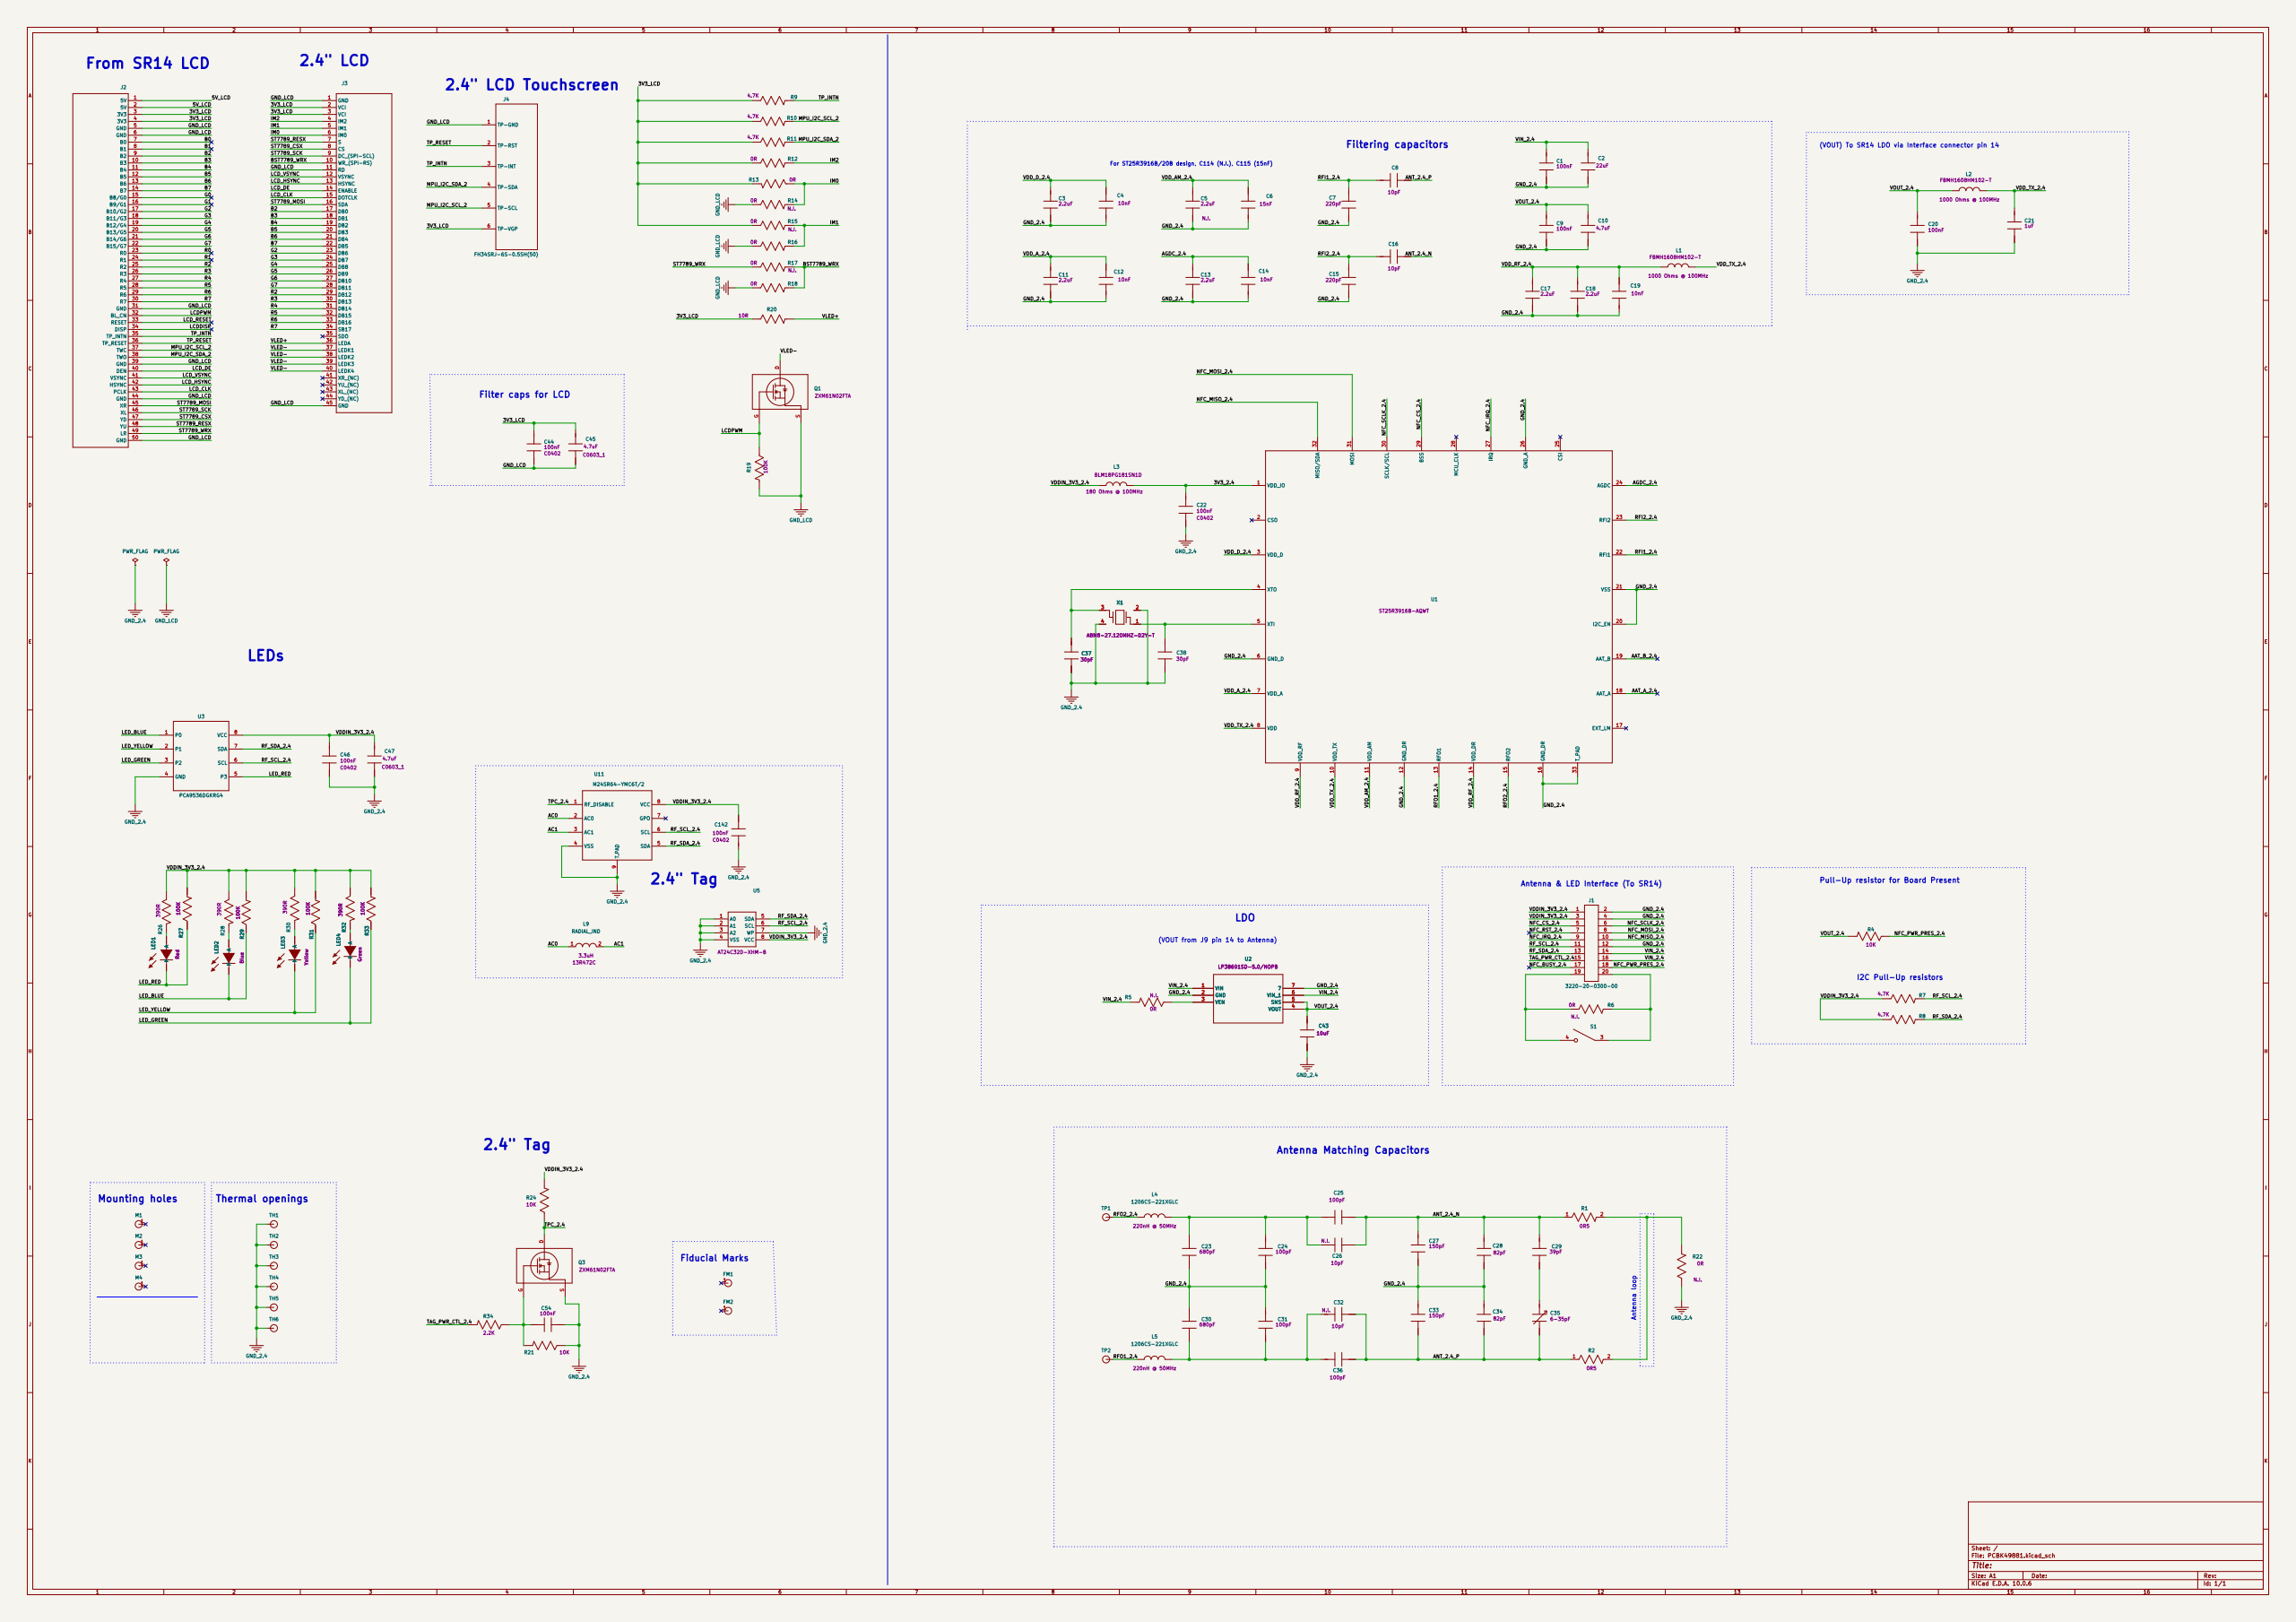Circuit board | KiCad | 113 parts | 116 nets
Bill of materials:
"Refs","Value","Footprint","Qty","DNP"
"C1,C4,C6,C7,C9,C12,C14,C15,C19-C34,C36-C38,C44,C46,C54,C142","CAP-SM","Capacitor_SMD:C_0402_1005Metric","31",""
"C2,C3,C5,C10,C11,C13,C17,C18,C43,C45,C47","CAP-SM","Capacitor_SMD:C_0603_1608Metric","11",""
"C8,C16","CAP","Capacitor_SMD:C_0402_1005Metric","2",""
"C35","TRIM_CAP","Library:TSC3S","1",""
"FM1,FM2","FM-40/80","Library:FM-40$2F$80","2",""
"J1","3220-20-0300-00","Library:3220-20-0300-00","1",""
"J2","LCM-50PIN-ANT","Library:LCD-50P-ANT","1",""
"J3","62684-452100ALF","Library:LCD-45P-0.5MM","1",""
"J4","FH34SRJ-6S-0.5SH(50)","Library:LCD-6P-0.5","1",""
"L1,L2","FBMH1608HM102","Library:FBMH1608HM102","2",""
"L3","IND-SMD","Library:INDC1608X90N","1",""
"L4,L5","1206CS-221XGLC","Library:1206CS-221XGLC","2",""
"L9","RADIAL_IND","Library:13R332C","1",""
"LED1-LED4","LED","Library:LED_0603_A","4",""
"M1-M4","MT_VIA","Library:MT-200$2F$125_VIA","4",""
"Q1,Q3","ZXM61N02FTA","Library:ZXM61N02F","2",""
"R1,R2","R1206","Resistor_SMD:R_0805_2012Metric","2",""
"R4-R19,R21,R22,R24,R26-R34","RES-SM","Resistor_SMD:R_0402_1005Metric","28",""
"R20","RES-SM","Resistor_SMD:R_0603_1608Metric","1",""
"S1","ESE13","Library:ESE13","1",""
"TH1-TH6","THERMAL_40/80","Library:THERMAL_40$2F$80","6",""
"TP1,TP2","TP","Library:TP_SM40","2",""
"U1","ST25R3920_1","Library:ST25R3920","1",""
"U2","LP38693SD-5.0/NOPB","Library:LP38693SD-5.0$2F$NOPB","1",""
"U3","PCA9536DGKRG4","Library:DGK8","1",""
"U5","CAT24C64","Library:TSSOP8","1",""
"U11","M24SR64-YMC6T/2","Library:UFDFPN8","1",""
"X1","ABM8-27.120MHZ-D2Y-T","Library:XTAL_3.6X2.8","1",""
Netlist (net: part-pin ...):
/3V3_2.4: C22-1 L3-1 U1-1
/3V3_LCD: C44-1 C45-1 J2-3 J2-4 J3-2 J3-3 J4-6 R9-1 R10-1 R11-1 R12-1 R13-2 R15-1 R20-1
/5V_LCD: J2-1 J2-2
/AAT_A_2.4: U1-18
/AAT_B_2.4: U1-19
/AC0: L9-1 U11-2
/AC1: L9-2 U11-3
/AGDC_2.4: C13-1 C14-2 U1-24
/ANT_2.4_N: C16-2 C25-2 C26-2 C27-1 C28-1 C29-1 R1-1
/ANT_2.4_P: C8-2 C32-2 C33-2 C34-2 C35-2 C36-2 R2-1
/B0: J2-7
/B1: J2-8
/B2: J2-9 J3-17
/B3: J2-10 J3-18
/B4: J2-11 J3-19
/B5: J2-12 J3-20
/B6: J2-13 J3-21
/B7: J2-14 J3-22
/BST7789_WRX: J3-10 R17-2 R18-2
/G0: J2-15
/G1: J2-16
/G2: J2-17 J3-23
/G3: J2-18 J3-24
/G4: J2-19 J3-25
/G5: J2-20 J3-26
/G6: J2-21 J3-27
/G7: J2-22 J3-28
/IM0: J3-6 R13-1 R14-2
/IM1: J3-5 R15-2 R16-2
/IM2: J3-4 R12-2
/LCDDISP: J2-34
/LCDPWM: J2-32 Q1-G R19-1
/LCD_CLK: J2-43 J3-15
/LCD_DE: J2-40 J3-14
/LCD_HSYNC: J2-42 J3-13
/LCD_RESET: J2-33
/LCD_VSYNC: J2-41 J3-12
/LED_BLUE: LED2-1 R29-1 U3-1
/LED_GREEN: LED4-1 R33-1 U3-3
/LED_RED: LED1-1 R27-1 U3-5
/LED_YELLOW: LED3-1 R31-1 U3-2
/MPU_I2C_SCL_2: J2-37 J4-5 R10-2
/MPU_I2C_SDA_2: J2-38 J4-4 R11-2
/NFC_BUSY_2.4: J1-17
/NFC_CS_2.4: J1-5 U1-29
/NFC_IRQ_2.4: J1-9 U1-27
/NFC_MISO_2.4: J1-10 U1-32
/NFC_MOSI_2.4: J1-8 U1-31
/NFC_PWR_PRES_2.4: J1-18 R4-1
/NFC_RST_2.4: J1-7
/NFC_SCLK_2.4: J1-6 U1-30
/R0: J2-23
/R1: J2-24
/R2: J2-25 J3-29
/R3: J2-26 J3-30
/R4: J2-27 J3-31
/R5: J2-28 J3-32
/R6: J2-29 J3-33
/R7: J2-30 J3-34
/RFI1_2.4: C7-1 C8-1 U1-22
/RFI2_2.4: C15-1 C16-1 U1-23
/RFO1_2.4: L5-1 TP2-1 U1-13
/RFO2_2.4: L4-1 TP1-1 U1-15
/RF_SCL_2.4: J1-11 R7-2 U3-6 U5-6 U11-6
/RF_SDA_2.4: J1-13 R8-2 U3-7 U5-5 U11-5
/ST7789_CSX: J2-47 J3-8
/ST7789_MOSI: J2-45 J3-16
/ST7789_RESX: J2-48 J3-7
/ST7789_SCK: J2-46 J3-9
/ST7789_WRX: J2-49 R17-1
/TAG_PWR_CTL_2.4: J1-15 R34-2
/TPC_2.4: Q3-D R24-1 U11-1
/TP_INTN: J2-35 J4-3 R9-2
/TP_RESET: J2-36 J4-2
/VDDIN_3V3_2.4: C46-1 C47-1 C142-2 J1-1 J1-3 L3-2 R7-1 R8-1 R24-2 R26-1 R27-2 R28-1 R29-2 R30-1 R31-2 R32-1 R33-2 U3-8 U5-8 U11-8
/VDD_AM_2.4: C5-1 C6-2 U1-11
/VDD_A_2.4: C11-1 C12-2 U1-7
/VDD_D_2.4: C3-1 C4-2 U1-3
/VDD_RF_2.4: C17-1 C18-1 C19-2 L1-1 U1-9 U1-14
/VDD_TX_2.4: C21-1 L1-2 L2-2 U1-8 U1-10
/VIN_2.4: C1-1 C2-1 J1-14 J1-16 R5-2 U2-1 U2-6
/VLED+: J3-36 R20-2
/VLED-: J3-37 J3-38 J3-39 J3-40 Q1-D
/VOUT_2.4: C9-1 C10-1 C20-1 C43-1 L2-1 R4-2 U2-4 U2-5
GND_2.4: C1-2 C2-2 C3-2 C4-1 C5-2 C6-1 C7-2 C9-2 C10-2 C11-2 C12-1 C13-2 C14-1 C15-2 C17-2 C18-2 C19-1 C20-2 C21-2 C22-2 C23-2 C24-2 C27-2 C28-2 C30-1 C31-1 C33-1 C34-1 C37-2 C38-2 C43-2 C46-2 C47-2 C54-1 C142-1 J1-2 J1-4 J1-12 Q3-S R21-1 R22-1 TH1-1 TH2-1 TH3-1 TH4-1 TH5-1 TH6-1 U1-6 U1-12 U1-16 U1-20 U1-21 U1-26 U1-33 U2-2 U2-7 U3-4 U5-1 U5-2 U5-3 U5-4 U5-7 U11-4 U11-9 X1-2 X1-4
GND_LCD: C44-2 C45-2 J2-5 J2-6 J2-31 J2-39 J2-44 J2-50 J3-1 J3-11 J3-45 J4-1 Q1-S R14-1 R16-1 R18-1 R19-2
Net-(C23-Pad1): C23-1 C24-1 C25-1 C26-1 L4-2
Net-(C29-Pad2): C29-2 C35-1
Net-(C30-Pad2): C30-2 C31-2 C32-1 C36-1 L5-2
Net-(C54-Pad2): C54-2 Q3-G R21-2 R34-1
Net-(J1-Pad19): J1-19 R6-1 S1-4
Net-(J1-Pad20): J1-20 R6-2 S1-3
Net-(LED1-A): LED1-2 R26-2
Net-(LED2-A): LED2-2 R28-2
Net-(LED3-A): LED3-2 R30-2
Net-(LED4-A): LED4-2 R32-2
Net-(R1-Pad2): R1-2 R2-2 R22-2
Net-(U1-XTI): C38-1 U1-5 X1-1
Net-(U1-XTO): C37-1 U1-4 X1-3
Net-(U2-VEN): R5-1 U2-3
unconnected-(FM1-TP-Pad1): FM1-1
unconnected-(FM2-TP-Pad1): FM2-1
unconnected-(J3-SDO-Pad35): J3-35
unconnected-(J3-XL_(NC)-Pad43): J3-43
unconnected-(J3-XR_(NC)-Pad41): J3-41
unconnected-(J3-YD_(NC)-Pad44): J3-44
unconnected-(J3-YU_(NC)-Pad42): J3-42
unconnected-(M1-TP-Pad1): M1-1
unconnected-(M2-TP-Pad1): M2-1
unconnected-(M3-TP-Pad1): M3-1
unconnected-(M4-TP-Pad1): M4-1
unconnected-(U1-CSI-Pad25): U1-25
unconnected-(U1-CSO-Pad2): U1-2
unconnected-(U1-EXT_LM-Pad17): U1-17
unconnected-(U1-MCU_CLK-Pad28): U1-28
unconnected-(U11-GPO-Pad7): U11-7